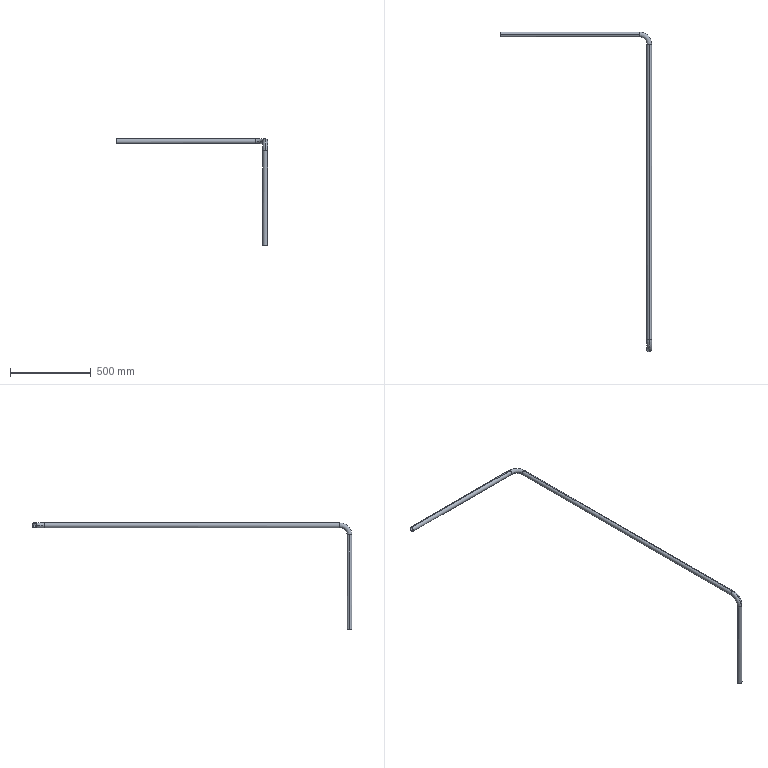Part | SolidWorks | features 3DProfileFeature 2, Sweep 1 | 1 solid | 22 faces | box 936.356 x 1980 x 658.195 mm | volume 609287 mm3 | cylinder 12 | torus 8 | plane 2 | commonest cylinder face diameters 26 x6 30 x6
STEP:
#1=CARTESIAN_POINT('',(750.,1143.697,-236.553));
#2=VERTEX_POINT('',#1);
#3=CARTESIAN_POINT('',(750.,1143.697,-210.553));
#4=VERTEX_POINT('',#3);
#5=CARTESIAN_POINT('',(750.,1143.697,-223.553));
#6=DIRECTION('',(0.,1.,0.));
#7=DIRECTION('',(0.,0.,-1.));
#8=AXIS2_PLACEMENT_3D('',#5,#6,#7);
#9=CIRCLE('',#8,13.);
#10=EDGE_CURVE('',#2,#4,#9,.T.);
#11=ORIENTED_EDGE('',*,*,#10,.T.);
#12=CARTESIAN_POINT('',(750.,1070.697,-283.553));
#13=VERTEX_POINT('',#12);
#14=CARTESIAN_POINT('',(750.,1143.697,-283.553));
#15=DIRECTION('',(1.,0.,0.));
#16=DIRECTION('',(0.,0.,-1.));
#17=AXIS2_PLACEMENT_3D('',#14,#15,#16);
#18=CIRCLE('',#17,73.);
#19=EDGE_CURVE('',#4,#13,#18,.T.);
#20=ORIENTED_EDGE('',*,*,#19,.T.);
#21=CARTESIAN_POINT('',(737.,1083.697,-283.553));
#22=VERTEX_POINT('',#21);
#23=CARTESIAN_POINT('',(750.,1083.697,-283.553));
#24=DIRECTION('',(0.,0.,1.));
#25=DIRECTION('',(0.,-1.,0.));
#26=AXIS2_PLACEMENT_3D('',#23,#24,#25);
#27=CIRCLE('',#26,13.);
#28=EDGE_CURVE('',#22,#13,#27,.T.);
#29=ORIENTED_EDGE('',*,*,#28,.F.);
#30=CARTESIAN_POINT('',(750.,1096.697,-283.553));
#31=VERTEX_POINT('',#30);
#32=CARTESIAN_POINT('',(750.,1083.697,-283.553));
#33=DIRECTION('',(0.,0.,1.));
#34=DIRECTION('',(0.,-1.,0.));
#35=AXIS2_PLACEMENT_3D('',#32,#33,#34);
#36=CIRCLE('',#35,13.);
#37=EDGE_CURVE('',#31,#22,#36,.T.);
#38=ORIENTED_EDGE('',*,*,#37,.F.);
#39=CARTESIAN_POINT('',(750.,1143.697,-283.553));
#40=DIRECTION('',(1.,0.,0.));
#41=DIRECTION('',(0.,0.,-1.));
#42=AXIS2_PLACEMENT_3D('',#39,#40,#41);
#43=CIRCLE('',#42,47.);
#44=EDGE_CURVE('',#2,#31,#43,.T.);
#45=ORIENTED_EDGE('',*,*,#44,.F.);
#46=EDGE_LOOP('',(#11,#20,#29,#38,#45));
#47=FACE_OUTER_BOUND('',#46,.T.);
#48=CARTESIAN_POINT('',(750.,1143.697,-283.553));
#49=DIRECTION('',(1.,0.,0.));
#50=DIRECTION('',(0.,0.,-1.));
#51=AXIS2_PLACEMENT_3D('',#48,#49,#50);
#52=TOROIDAL_SURFACE('',#51,60.,13.);
#53=ADVANCED_FACE('',(#47),#52,.F.);
#54=CARTESIAN_POINT('',(690.,3033.901,-210.553));
#55=VERTEX_POINT('',#54);
#56=CARTESIAN_POINT('',(690.,3046.901,-223.553));
#57=VERTEX_POINT('',#56);
#58=CARTESIAN_POINT('',(690.,3033.901,-223.553));
#59=DIRECTION('',(-1.,0.,0.));
#60=DIRECTION('',(0.,0.,-1.));
#61=AXIS2_PLACEMENT_3D('',#58,#59,#60);
#62=CIRCLE('',#61,13.);
#63=EDGE_CURVE('',#55,#57,#62,.T.);
#64=ORIENTED_EDGE('',*,*,#63,.T.);
#65=CARTESIAN_POINT('',(763.,2973.901,-223.553));
#66=VERTEX_POINT('',#65);
#67=CARTESIAN_POINT('',(690.,2973.901,-223.553));
#68=DIRECTION('',(0.,0.,-1.));
#69=DIRECTION('',(-1.,0.,0.));
#70=AXIS2_PLACEMENT_3D('',#67,#68,#69);
#71=CIRCLE('',#70,73.);
#72=EDGE_CURVE('',#57,#66,#71,.T.);
#73=ORIENTED_EDGE('',*,*,#72,.T.);
#74=CARTESIAN_POINT('',(750.,2973.901,-210.553));
#75=VERTEX_POINT('',#74);
#76=CARTESIAN_POINT('',(750.,2973.901,-223.553));
#77=DIRECTION('',(0.,1.,0.));
#78=DIRECTION('',(-1.,0.,0.));
#79=AXIS2_PLACEMENT_3D('',#76,#77,#78);
#80=CIRCLE('',#79,13.);
#81=EDGE_CURVE('',#75,#66,#80,.T.);
#82=ORIENTED_EDGE('',*,*,#81,.F.);
#83=CARTESIAN_POINT('',(737.,2973.901,-223.553));
#84=VERTEX_POINT('',#83);
#85=CARTESIAN_POINT('',(750.,2973.901,-223.553));
#86=DIRECTION('',(0.,1.,0.));
#87=DIRECTION('',(-1.,0.,0.));
#88=AXIS2_PLACEMENT_3D('',#85,#86,#87);
#89=CIRCLE('',#88,13.);
#90=EDGE_CURVE('',#84,#75,#89,.T.);
#91=ORIENTED_EDGE('',*,*,#90,.F.);
#92=CARTESIAN_POINT('',(690.,3020.901,-223.553));
#93=VERTEX_POINT('',#92);
#94=CARTESIAN_POINT('',(690.,2973.901,-223.553));
#95=DIRECTION('',(0.,0.,-1.));
#96=DIRECTION('',(-1.,0.,0.));
#97=AXIS2_PLACEMENT_3D('',#94,#95,#96);
#98=CIRCLE('',#97,47.);
#99=EDGE_CURVE('',#93,#84,#98,.T.);
#100=ORIENTED_EDGE('',*,*,#99,.F.);
#101=CARTESIAN_POINT('',(690.,3033.901,-223.553));
#102=DIRECTION('',(-1.,0.,0.));
#103=DIRECTION('',(0.,0.,-1.));
#104=AXIS2_PLACEMENT_3D('',#101,#102,#103);
#105=CIRCLE('',#104,13.);
#106=EDGE_CURVE('',#93,#55,#105,.T.);
#107=ORIENTED_EDGE('',*,*,#106,.T.);
#108=EDGE_LOOP('',(#64,#73,#82,#91,#100,#107));
#109=FACE_OUTER_BOUND('',#108,.T.);
#110=CARTESIAN_POINT('',(690.,2973.901,-223.553));
#111=DIRECTION('',(0.,0.,-1.));
#112=DIRECTION('',(-1.,0.,0.));
#113=AXIS2_PLACEMENT_3D('',#110,#111,#112);
#114=TOROIDAL_SURFACE('',#113,60.,13.);
#115=ADVANCED_FACE('',(#109),#114,.F.);
#116=CARTESIAN_POINT('',(750.,1143.697,-208.553));
#117=VERTEX_POINT('',#116);
#118=CARTESIAN_POINT('',(750.,1143.697,-238.553));
#119=VERTEX_POINT('',#118);
#120=CARTESIAN_POINT('',(750.,1143.697,-223.553));
#121=DIRECTION('',(0.,1.,0.));
#122=DIRECTION('',(1.,0.,0.));
#123=AXIS2_PLACEMENT_3D('',#120,#121,#122);
#124=CIRCLE('',#123,15.);
#125=EDGE_CURVE('',#117,#119,#124,.T.);
#126=ORIENTED_EDGE('',*,*,#125,.F.);
#127=CARTESIAN_POINT('',(750.,1068.697,-283.553));
#128=VERTEX_POINT('',#127);
#129=CARTESIAN_POINT('',(750.,1143.697,-283.553));
#130=DIRECTION('',(1.,0.,0.));
#131=DIRECTION('',(0.,0.,-1.));
#132=AXIS2_PLACEMENT_3D('',#129,#130,#131);
#133=CIRCLE('',#132,75.);
#134=EDGE_CURVE('',#117,#128,#133,.T.);
#135=ORIENTED_EDGE('',*,*,#134,.T.);
#136=CARTESIAN_POINT('',(765.,1083.697,-283.553));
#137=VERTEX_POINT('',#136);
#138=CARTESIAN_POINT('',(750.,1083.697,-283.553));
#139=DIRECTION('',(0.,0.,1.));
#140=DIRECTION('',(1.,0.,0.));
#141=AXIS2_PLACEMENT_3D('',#138,#139,#140);
#142=CIRCLE('',#141,15.);
#143=EDGE_CURVE('',#128,#137,#142,.T.);
#144=ORIENTED_EDGE('',*,*,#143,.T.);
#145=CARTESIAN_POINT('',(750.,1098.697,-283.553));
#146=VERTEX_POINT('',#145);
#147=CARTESIAN_POINT('',(750.,1083.697,-283.553));
#148=DIRECTION('',(0.,0.,1.));
#149=DIRECTION('',(1.,0.,0.));
#150=AXIS2_PLACEMENT_3D('',#147,#148,#149);
#151=CIRCLE('',#150,15.);
#152=EDGE_CURVE('',#137,#146,#151,.T.);
#153=ORIENTED_EDGE('',*,*,#152,.T.);
#154=CARTESIAN_POINT('',(750.,1143.697,-283.553));
#155=DIRECTION('',(1.,0.,0.));
#156=DIRECTION('',(0.,0.,-1.));
#157=AXIS2_PLACEMENT_3D('',#154,#155,#156);
#158=CIRCLE('',#157,45.);
#159=EDGE_CURVE('',#119,#146,#158,.T.);
#160=ORIENTED_EDGE('',*,*,#159,.F.);
#161=EDGE_LOOP('',(#126,#135,#144,#153,#160));
#162=FACE_OUTER_BOUND('',#161,.T.);
#163=CARTESIAN_POINT('',(750.,1143.697,-283.553));
#164=DIRECTION('',(1.,0.,0.));
#165=DIRECTION('',(0.,0.,-1.));
#166=AXIS2_PLACEMENT_3D('',#163,#164,#165);
#167=TOROIDAL_SURFACE('',#166,60.,15.);
#168=ADVANCED_FACE('',(#162),#167,.T.);
#169=CARTESIAN_POINT('',(690.,3048.901,-223.553));
#170=VERTEX_POINT('',#169);
#171=CARTESIAN_POINT('',(690.,3033.901,-238.553));
#172=VERTEX_POINT('',#171);
#173=CARTESIAN_POINT('',(690.,3033.901,-223.553));
#174=DIRECTION('',(-1.,0.,0.));
#175=DIRECTION('',(0.,1.,0.));
#176=AXIS2_PLACEMENT_3D('',#173,#174,#175);
#177=CIRCLE('',#176,15.);
#178=EDGE_CURVE('',#170,#172,#177,.T.);
#179=ORIENTED_EDGE('',*,*,#178,.F.);
#180=CARTESIAN_POINT('',(765.,2973.901,-223.553));
#181=VERTEX_POINT('',#180);
#182=CARTESIAN_POINT('',(690.,2973.901,-223.553));
#183=DIRECTION('',(0.,0.,-1.));
#184=DIRECTION('',(-1.,0.,0.));
#185=AXIS2_PLACEMENT_3D('',#182,#183,#184);
#186=CIRCLE('',#185,75.);
#187=EDGE_CURVE('',#170,#181,#186,.T.);
#188=ORIENTED_EDGE('',*,*,#187,.T.);
#189=CARTESIAN_POINT('',(750.,2973.901,-238.553));
#190=VERTEX_POINT('',#189);
#191=CARTESIAN_POINT('',(750.,2973.901,-223.553));
#192=DIRECTION('',(0.,1.,0.));
#193=DIRECTION('',(1.,0.,0.));
#194=AXIS2_PLACEMENT_3D('',#191,#192,#193);
#195=CIRCLE('',#194,15.);
#196=EDGE_CURVE('',#181,#190,#195,.T.);
#197=ORIENTED_EDGE('',*,*,#196,.T.);
#198=CARTESIAN_POINT('',(735.,2973.901,-223.553));
#199=VERTEX_POINT('',#198);
#200=CARTESIAN_POINT('',(750.,2973.901,-223.553));
#201=DIRECTION('',(0.,1.,0.));
#202=DIRECTION('',(1.,0.,0.));
#203=AXIS2_PLACEMENT_3D('',#200,#201,#202);
#204=CIRCLE('',#203,15.);
#205=EDGE_CURVE('',#190,#199,#204,.T.);
#206=ORIENTED_EDGE('',*,*,#205,.T.);
#207=CARTESIAN_POINT('',(690.,3018.901,-223.553));
#208=VERTEX_POINT('',#207);
#209=CARTESIAN_POINT('',(690.,2973.901,-223.553));
#210=DIRECTION('',(0.,0.,-1.));
#211=DIRECTION('',(-1.,0.,0.));
#212=AXIS2_PLACEMENT_3D('',#209,#210,#211);
#213=CIRCLE('',#212,45.);
#214=EDGE_CURVE('',#208,#199,#213,.T.);
#215=ORIENTED_EDGE('',*,*,#214,.F.);
#216=CARTESIAN_POINT('',(690.,3033.901,-223.553));
#217=DIRECTION('',(-1.,0.,0.));
#218=DIRECTION('',(0.,1.,0.));
#219=AXIS2_PLACEMENT_3D('',#216,#217,#218);
#220=CIRCLE('',#219,15.);
#221=EDGE_CURVE('',#172,#208,#220,.T.);
#222=ORIENTED_EDGE('',*,*,#221,.F.);
#223=EDGE_LOOP('',(#179,#188,#197,#206,#215,#222));
#224=FACE_OUTER_BOUND('',#223,.T.);
#225=CARTESIAN_POINT('',(690.,2973.901,-223.553));
#226=DIRECTION('',(0.,0.,-1.));
#227=DIRECTION('',(-1.,0.,0.));
#228=AXIS2_PLACEMENT_3D('',#225,#226,#227);
#229=TOROIDAL_SURFACE('',#228,60.,15.);
#230=ADVANCED_FACE('',(#224),#229,.T.);
#231=ORIENTED_EDGE('',*,*,#28,.T.);
#232=CARTESIAN_POINT('',(763.,1083.697,-283.553));
#233=VERTEX_POINT('',#232);
#234=CARTESIAN_POINT('',(750.,1083.697,-283.553));
#235=DIRECTION('',(0.,0.,1.));
#236=DIRECTION('',(0.,-1.,0.));
#237=AXIS2_PLACEMENT_3D('',#234,#235,#236);
#238=CIRCLE('',#237,13.);
#239=EDGE_CURVE('',#13,#233,#238,.T.);
#240=ORIENTED_EDGE('',*,*,#239,.T.);
#241=CARTESIAN_POINT('',(763.,1083.697,-866.748));
#242=VERTEX_POINT('',#241);
#243=CARTESIAN_POINT('',(763.,1083.697,-283.553));
#244=DIRECTION('',(0.,0.,-1.));
#245=VECTOR('',#244,1000.);
#246=LINE('',#243,#245);
#247=EDGE_CURVE('',#233,#242,#246,.T.);
#248=ORIENTED_EDGE('',*,*,#247,.T.);
#249=CARTESIAN_POINT('',(737.,1083.697,-866.748));
#250=VERTEX_POINT('',#249);
#251=CARTESIAN_POINT('',(750.,1083.697,-866.748));
#252=DIRECTION('',(0.,0.,1.));
#253=DIRECTION('',(1.,0.,0.));
#254=AXIS2_PLACEMENT_3D('',#251,#252,#253);
#255=CIRCLE('',#254,13.);
#256=EDGE_CURVE('',#250,#242,#255,.T.);
#257=ORIENTED_EDGE('',*,*,#256,.F.);
#258=CARTESIAN_POINT('',(737.,1083.697,-283.553));
#259=DIRECTION('',(0.,0.,-1.));
#260=VECTOR('',#259,1000.);
#261=LINE('',#258,#260);
#262=EDGE_CURVE('',#22,#250,#261,.T.);
#263=ORIENTED_EDGE('',*,*,#262,.F.);
#264=EDGE_LOOP('',(#231,#240,#248,#257,#263));
#265=FACE_OUTER_BOUND('',#264,.T.);
#266=CARTESIAN_POINT('',(750.,1083.697,-283.553));
#267=DIRECTION('',(0.,0.,-1.));
#268=DIRECTION('',(-1.,0.,0.));
#269=AXIS2_PLACEMENT_3D('',#266,#267,#268);
#270=CYLINDRICAL_SURFACE('',#269,13.);
#271=ADVANCED_FACE('',(#265),#270,.F.);
#272=CARTESIAN_POINT('',(750.,2973.901,-236.553));
#273=VERTEX_POINT('',#272);
#274=CARTESIAN_POINT('',(750.,2973.901,-223.553));
#275=DIRECTION('',(0.,1.,0.));
#276=DIRECTION('',(-1.,0.,0.));
#277=AXIS2_PLACEMENT_3D('',#274,#275,#276);
#278=CIRCLE('',#277,13.);
#279=EDGE_CURVE('',#273,#84,#278,.T.);
#280=ORIENTED_EDGE('',*,*,#279,.T.);
#281=ORIENTED_EDGE('',*,*,#90,.T.);
#282=CARTESIAN_POINT('',(750.,2973.901,-210.553));
#283=DIRECTION('',(0.,-1.,0.));
#284=VECTOR('',#283,1000.);
#285=LINE('',#282,#284);
#286=EDGE_CURVE('',#75,#4,#285,.T.);
#287=ORIENTED_EDGE('',*,*,#286,.T.);
#288=ORIENTED_EDGE('',*,*,#10,.F.);
#289=CARTESIAN_POINT('',(750.,2973.901,-236.553));
#290=DIRECTION('',(0.,-1.,0.));
#291=VECTOR('',#290,1000.);
#292=LINE('',#289,#291);
#293=EDGE_CURVE('',#273,#2,#292,.T.);
#294=ORIENTED_EDGE('',*,*,#293,.F.);
#295=EDGE_LOOP('',(#280,#281,#287,#288,#294));
#296=FACE_OUTER_BOUND('',#295,.T.);
#297=CARTESIAN_POINT('',(750.,2973.901,-223.553));
#298=DIRECTION('',(0.,-1.,0.));
#299=DIRECTION('',(0.,0.,-1.));
#300=AXIS2_PLACEMENT_3D('',#297,#298,#299);
#301=CYLINDRICAL_SURFACE('',#300,13.);
#302=ADVANCED_FACE('',(#296),#301,.F.);
#303=CARTESIAN_POINT('',(-171.356,3033.901,-236.553));
#304=VERTEX_POINT('',#303);
#305=CARTESIAN_POINT('',(-171.356,3033.901,-210.553));
#306=VERTEX_POINT('',#305);
#307=CARTESIAN_POINT('',(-171.356,3033.901,-223.553));
#308=DIRECTION('',(-1.,0.,0.));
#309=DIRECTION('',(0.,0.,1.));
#310=AXIS2_PLACEMENT_3D('',#307,#308,#309);
#311=CIRCLE('',#310,13.);
#312=EDGE_CURVE('',#304,#306,#311,.T.);
#313=ORIENTED_EDGE('',*,*,#312,.T.);
#314=CARTESIAN_POINT('',(-171.356,3033.901,-210.553));
#315=DIRECTION('',(1.,0.,0.));
#316=VECTOR('',#315,1000.);
#317=LINE('',#314,#316);
#318=EDGE_CURVE('',#306,#55,#317,.T.);
#319=ORIENTED_EDGE('',*,*,#318,.T.);
#320=ORIENTED_EDGE('',*,*,#106,.F.);
#321=CARTESIAN_POINT('',(690.,3033.901,-236.553));
#322=VERTEX_POINT('',#321);
#323=CARTESIAN_POINT('',(690.,3033.901,-223.553));
#324=DIRECTION('',(-1.,0.,0.));
#325=DIRECTION('',(0.,0.,-1.));
#326=AXIS2_PLACEMENT_3D('',#323,#324,#325);
#327=CIRCLE('',#326,13.);
#328=EDGE_CURVE('',#322,#93,#327,.T.);
#329=ORIENTED_EDGE('',*,*,#328,.F.);
#330=CARTESIAN_POINT('',(-171.356,3033.901,-236.553));
#331=DIRECTION('',(1.,0.,0.));
#332=VECTOR('',#331,1000.);
#333=LINE('',#330,#332);
#334=EDGE_CURVE('',#304,#322,#333,.T.);
#335=ORIENTED_EDGE('',*,*,#334,.F.);
#336=EDGE_LOOP('',(#313,#319,#320,#329,#335));
#337=FACE_OUTER_BOUND('',#336,.T.);
#338=CARTESIAN_POINT('',(-171.356,3033.901,-223.553));
#339=DIRECTION('',(1.,0.,0.));
#340=DIRECTION('',(0.,0.,-1.));
#341=AXIS2_PLACEMENT_3D('',#338,#339,#340);
#342=CYLINDRICAL_SURFACE('',#341,13.);
#343=ADVANCED_FACE('',(#337),#342,.F.);
#344=ORIENTED_EDGE('',*,*,#152,.F.);
#345=CARTESIAN_POINT('',(765.,1083.697,-866.748));
#346=VERTEX_POINT('',#345);
#347=CARTESIAN_POINT('',(765.,1083.697,-283.553));
#348=DIRECTION('',(0.,0.,-1.));
#349=VECTOR('',#348,1000.);
#350=LINE('',#347,#349);
#351=EDGE_CURVE('',#137,#346,#350,.T.);
#352=ORIENTED_EDGE('',*,*,#351,.T.);
#353=CARTESIAN_POINT('',(735.,1083.697,-866.748));
#354=VERTEX_POINT('',#353);
#355=CARTESIAN_POINT('',(750.,1083.697,-866.748));
#356=DIRECTION('',(0.,0.,1.));
#357=DIRECTION('',(1.,0.,0.));
#358=AXIS2_PLACEMENT_3D('',#355,#356,#357);
#359=CIRCLE('',#358,15.);
#360=EDGE_CURVE('',#346,#354,#359,.T.);
#361=ORIENTED_EDGE('',*,*,#360,.T.);
#362=CARTESIAN_POINT('',(735.,1083.697,-283.553));
#363=VERTEX_POINT('',#362);
#364=CARTESIAN_POINT('',(735.,1083.697,-283.553));
#365=DIRECTION('',(0.,0.,-1.));
#366=VECTOR('',#365,1000.);
#367=LINE('',#364,#366);
#368=EDGE_CURVE('',#363,#354,#367,.T.);
#369=ORIENTED_EDGE('',*,*,#368,.F.);
#370=CARTESIAN_POINT('',(750.,1083.697,-283.553));
#371=DIRECTION('',(0.,0.,1.));
#372=DIRECTION('',(1.,0.,0.));
#373=AXIS2_PLACEMENT_3D('',#370,#371,#372);
#374=CIRCLE('',#373,15.);
#375=EDGE_CURVE('',#146,#363,#374,.T.);
#376=ORIENTED_EDGE('',*,*,#375,.F.);
#377=EDGE_LOOP('',(#344,#352,#361,#369,#376));
#378=FACE_OUTER_BOUND('',#377,.T.);
#379=CARTESIAN_POINT('',(750.,1083.697,-283.553));
#380=DIRECTION('',(0.,0.,-1.));
#381=DIRECTION('',(-1.,0.,0.));
#382=AXIS2_PLACEMENT_3D('',#379,#380,#381);
#383=CYLINDRICAL_SURFACE('',#382,15.);
#384=ADVANCED_FACE('',(#378),#383,.T.);
#385=CARTESIAN_POINT('',(750.,2973.901,-208.553));
#386=VERTEX_POINT('',#385);
#387=CARTESIAN_POINT('',(750.,2973.901,-223.553));
#388=DIRECTION('',(0.,1.,0.));
#389=DIRECTION('',(1.,0.,0.));
#390=AXIS2_PLACEMENT_3D('',#387,#388,#389);
#391=CIRCLE('',#390,15.);
#392=EDGE_CURVE('',#386,#181,#391,.T.);
#393=ORIENTED_EDGE('',*,*,#392,.F.);
#394=CARTESIAN_POINT('',(750.,2973.901,-208.553));
#395=DIRECTION('',(0.,-1.,0.));
#396=VECTOR('',#395,1000.);
#397=LINE('',#394,#396);
#398=EDGE_CURVE('',#386,#117,#397,.T.);
#399=ORIENTED_EDGE('',*,*,#398,.T.);
#400=ORIENTED_EDGE('',*,*,#125,.T.);
#401=CARTESIAN_POINT('',(750.,2973.901,-238.553));
#402=DIRECTION('',(0.,-1.,0.));
#403=VECTOR('',#402,1000.);
#404=LINE('',#401,#403);
#405=EDGE_CURVE('',#190,#119,#404,.T.);
#406=ORIENTED_EDGE('',*,*,#405,.F.);
#407=ORIENTED_EDGE('',*,*,#196,.F.);
#408=EDGE_LOOP('',(#393,#399,#400,#406,#407));
#409=FACE_OUTER_BOUND('',#408,.T.);
#410=CARTESIAN_POINT('',(750.,2973.901,-223.553));
#411=DIRECTION('',(0.,-1.,0.));
#412=DIRECTION('',(0.,0.,-1.));
#413=AXIS2_PLACEMENT_3D('',#410,#411,#412);
#414=CYLINDRICAL_SURFACE('',#413,15.);
#415=ADVANCED_FACE('',(#409),#414,.T.);
#416=CARTESIAN_POINT('',(-171.356,3033.901,-208.553));
#417=VERTEX_POINT('',#416);
#418=CARTESIAN_POINT('',(-171.356,3033.901,-238.553));
#419=VERTEX_POINT('',#418);
#420=CARTESIAN_POINT('',(-171.356,3033.901,-223.553));
#421=DIRECTION('',(-1.,0.,0.));
#422=DIRECTION('',(0.,1.,0.));
#423=AXIS2_PLACEMENT_3D('',#420,#421,#422);
#424=CIRCLE('',#423,15.);
#425=EDGE_CURVE('',#417,#419,#424,.T.);
#426=ORIENTED_EDGE('',*,*,#425,.F.);
#427=CARTESIAN_POINT('',(690.,3033.901,-208.553));
#428=VERTEX_POINT('',#427);
#429=CARTESIAN_POINT('',(-171.356,3033.901,-208.553));
#430=DIRECTION('',(1.,0.,0.));
#431=VECTOR('',#430,1000.);
#432=LINE('',#429,#431);
#433=EDGE_CURVE('',#417,#428,#432,.T.);
#434=ORIENTED_EDGE('',*,*,#433,.T.);
#435=CARTESIAN_POINT('',(690.,3033.901,-223.553));
#436=DIRECTION('',(-1.,0.,0.));
#437=DIRECTION('',(0.,1.,0.));
#438=AXIS2_PLACEMENT_3D('',#435,#436,#437);
#439=CIRCLE('',#438,15.);
#440=EDGE_CURVE('',#428,#170,#439,.T.);
#441=ORIENTED_EDGE('',*,*,#440,.T.);
#442=ORIENTED_EDGE('',*,*,#178,.T.);
#443=CARTESIAN_POINT('',(-171.356,3033.901,-238.553));
#444=DIRECTION('',(1.,0.,0.));
#445=VECTOR('',#444,1000.);
#446=LINE('',#443,#445);
#447=EDGE_CURVE('',#419,#172,#446,.T.);
#448=ORIENTED_EDGE('',*,*,#447,.F.);
#449=EDGE_LOOP('',(#426,#434,#441,#442,#448));
#450=FACE_OUTER_BOUND('',#449,.T.);
#451=CARTESIAN_POINT('',(-171.356,3033.901,-223.553));
#452=DIRECTION('',(1.,0.,0.));
#453=DIRECTION('',(0.,0.,-1.));
#454=AXIS2_PLACEMENT_3D('',#451,#452,#453);
#455=CYLINDRICAL_SURFACE('',#454,15.);
#456=ADVANCED_FACE('',(#450),#455,.T.);
#457=ORIENTED_EDGE('',*,*,#351,.F.);
#458=ORIENTED_EDGE('',*,*,#143,.F.);
#459=CARTESIAN_POINT('',(750.,1083.697,-283.553));
#460=DIRECTION('',(0.,0.,1.));
#461=DIRECTION('',(1.,0.,0.));
#462=AXIS2_PLACEMENT_3D('',#459,#460,#461);
#463=CIRCLE('',#462,15.);
#464=EDGE_CURVE('',#363,#128,#463,.T.);
#465=ORIENTED_EDGE('',*,*,#464,.F.);
#466=ORIENTED_EDGE('',*,*,#368,.T.);
#467=CARTESIAN_POINT('',(750.,1083.697,-866.748));
#468=DIRECTION('',(0.,0.,1.));
#469=DIRECTION('',(1.,0.,0.));
#470=AXIS2_PLACEMENT_3D('',#467,#468,#469);
#471=CIRCLE('',#470,15.);
#472=EDGE_CURVE('',#354,#346,#471,.T.);
#473=ORIENTED_EDGE('',*,*,#472,.T.);
#474=EDGE_LOOP('',(#457,#458,#465,#466,#473));
#475=FACE_OUTER_BOUND('',#474,.T.);
#476=CARTESIAN_POINT('',(750.,1083.697,-283.553));
#477=DIRECTION('',(0.,0.,-1.));
#478=DIRECTION('',(-1.,0.,0.));
#479=AXIS2_PLACEMENT_3D('',#476,#477,#478);
#480=CYLINDRICAL_SURFACE('',#479,15.);
#481=ADVANCED_FACE('',(#475),#480,.T.);
#482=ORIENTED_EDGE('',*,*,#134,.F.);
#483=CARTESIAN_POINT('',(750.,1143.697,-223.553));
#484=DIRECTION('',(0.,1.,0.));
#485=DIRECTION('',(1.,0.,0.));
#486=AXIS2_PLACEMENT_3D('',#483,#484,#485);
#487=CIRCLE('',#486,15.);
#488=EDGE_CURVE('',#119,#117,#487,.T.);
#489=ORIENTED_EDGE('',*,*,#488,.F.);
#490=ORIENTED_EDGE('',*,*,#159,.T.);
#491=ORIENTED_EDGE('',*,*,#375,.T.);
#492=ORIENTED_EDGE('',*,*,#464,.T.);
#493=EDGE_LOOP('',(#482,#489,#490,#491,#492));
#494=FACE_OUTER_BOUND('',#493,.T.);
#495=CARTESIAN_POINT('',(750.,1143.697,-283.553));
#496=DIRECTION('',(1.,0.,0.));
#497=DIRECTION('',(0.,0.,-1.));
#498=AXIS2_PLACEMENT_3D('',#495,#496,#497);
#499=TOROIDAL_SURFACE('',#498,60.,15.);
#500=ADVANCED_FACE('',(#494),#499,.T.);
#501=ORIENTED_EDGE('',*,*,#398,.F.);
#502=CARTESIAN_POINT('',(750.,2973.901,-223.553));
#503=DIRECTION('',(0.,1.,0.));
#504=DIRECTION('',(1.,0.,0.));
#505=AXIS2_PLACEMENT_3D('',#502,#503,#504);
#506=CIRCLE('',#505,15.);
#507=EDGE_CURVE('',#199,#386,#506,.T.);
#508=ORIENTED_EDGE('',*,*,#507,.F.);
#509=ORIENTED_EDGE('',*,*,#205,.F.);
#510=ORIENTED_EDGE('',*,*,#405,.T.);
#511=ORIENTED_EDGE('',*,*,#488,.T.);
#512=EDGE_LOOP('',(#501,#508,#509,#510,#511));
#513=FACE_OUTER_BOUND('',#512,.T.);
#514=CARTESIAN_POINT('',(750.,2973.901,-223.553));
#515=DIRECTION('',(0.,-1.,0.));
#516=DIRECTION('',(0.,0.,-1.));
#517=AXIS2_PLACEMENT_3D('',#514,#515,#516);
#518=CYLINDRICAL_SURFACE('',#517,15.);
#519=ADVANCED_FACE('',(#513),#518,.T.);
#520=ORIENTED_EDGE('',*,*,#187,.F.);
#521=ORIENTED_EDGE('',*,*,#440,.F.);
#522=CARTESIAN_POINT('',(690.,3033.901,-223.553));
#523=DIRECTION('',(-1.,0.,0.));
#524=DIRECTION('',(0.,1.,0.));
#525=AXIS2_PLACEMENT_3D('',#522,#523,#524);
#526=CIRCLE('',#525,15.);
#527=EDGE_CURVE('',#208,#428,#526,.T.);
#528=ORIENTED_EDGE('',*,*,#527,.F.);
#529=ORIENTED_EDGE('',*,*,#214,.T.);
#530=ORIENTED_EDGE('',*,*,#507,.T.);
#531=ORIENTED_EDGE('',*,*,#392,.T.);
#532=EDGE_LOOP('',(#520,#521,#528,#529,#530,#531));
#533=FACE_OUTER_BOUND('',#532,.T.);
#534=CARTESIAN_POINT('',(690.,2973.901,-223.553));
#535=DIRECTION('',(0.,0.,-1.));
#536=DIRECTION('',(-1.,0.,0.));
#537=AXIS2_PLACEMENT_3D('',#534,#535,#536);
#538=TOROIDAL_SURFACE('',#537,60.,15.);
#539=ADVANCED_FACE('',(#533),#538,.T.);
#540=ORIENTED_EDGE('',*,*,#433,.F.);
#541=CARTESIAN_POINT('',(-171.356,3033.901,-223.553));
#542=DIRECTION('',(-1.,0.,0.));
#543=DIRECTION('',(0.,1.,0.));
#544=AXIS2_PLACEMENT_3D('',#541,#542,#543);
#545=CIRCLE('',#544,15.);
#546=EDGE_CURVE('',#419,#417,#545,.T.);
#547=ORIENTED_EDGE('',*,*,#546,.F.);
#548=ORIENTED_EDGE('',*,*,#447,.T.);
#549=ORIENTED_EDGE('',*,*,#221,.T.);
#550=ORIENTED_EDGE('',*,*,#527,.T.);
#551=EDGE_LOOP('',(#540,#547,#548,#549,#550));
#552=FACE_OUTER_BOUND('',#551,.T.);
#553=CARTESIAN_POINT('',(-171.356,3033.901,-223.553));
#554=DIRECTION('',(1.,0.,0.));
#555=DIRECTION('',(0.,0.,-1.));
#556=AXIS2_PLACEMENT_3D('',#553,#554,#555);
#557=CYLINDRICAL_SURFACE('',#556,15.);
#558=ADVANCED_FACE('',(#552),#557,.T.);
#559=ORIENTED_EDGE('',*,*,#256,.T.);
#560=CARTESIAN_POINT('',(750.,1083.697,-866.748));
#561=DIRECTION('',(0.,0.,1.));
#562=DIRECTION('',(1.,0.,0.));
#563=AXIS2_PLACEMENT_3D('',#560,#561,#562);
#564=CIRCLE('',#563,13.);
#565=EDGE_CURVE('',#242,#250,#564,.T.);
#566=ORIENTED_EDGE('',*,*,#565,.T.);
#567=EDGE_LOOP('',(#559,#566));
#568=FACE_BOUND('',#567,.T.);
#569=ORIENTED_EDGE('',*,*,#472,.F.);
#570=ORIENTED_EDGE('',*,*,#360,.F.);
#571=EDGE_LOOP('',(#569,#570));
#572=FACE_OUTER_BOUND('',#571,.T.);
#573=CARTESIAN_POINT('',(750.,1083.697,-866.748));
#574=DIRECTION('',(0.,0.,1.));
#575=DIRECTION('',(1.,0.,0.));
#576=AXIS2_PLACEMENT_3D('',#573,#574,#575);
#577=PLANE('',#576);
#578=ADVANCED_FACE('',(#568,#572),#577,.F.);
#579=ORIENTED_EDGE('',*,*,#312,.F.);
#580=CARTESIAN_POINT('',(-171.356,3033.901,-223.553));
#581=DIRECTION('',(-1.,0.,0.));
#582=DIRECTION('',(0.,0.,1.));
#583=AXIS2_PLACEMENT_3D('',#580,#581,#582);
#584=CIRCLE('',#583,13.);
#585=EDGE_CURVE('',#306,#304,#584,.T.);
#586=ORIENTED_EDGE('',*,*,#585,.F.);
#587=EDGE_LOOP('',(#579,#586));
#588=FACE_BOUND('',#587,.T.);
#589=ORIENTED_EDGE('',*,*,#546,.T.);
#590=ORIENTED_EDGE('',*,*,#425,.T.);
#591=EDGE_LOOP('',(#589,#590));
#592=FACE_OUTER_BOUND('',#591,.T.);
#593=CARTESIAN_POINT('',(-171.356,3033.901,-223.553));
#594=DIRECTION('',(-1.,0.,0.));
#595=DIRECTION('',(0.,1.,0.));
#596=AXIS2_PLACEMENT_3D('',#593,#594,#595);
#597=PLANE('',#596);
#598=ADVANCED_FACE('',(#588,#592),#597,.T.);
#599=ORIENTED_EDGE('',*,*,#247,.F.);
#600=CARTESIAN_POINT('',(750.,1083.697,-283.553));
#601=DIRECTION('',(0.,0.,1.));
#602=DIRECTION('',(0.,-1.,0.));
#603=AXIS2_PLACEMENT_3D('',#600,#601,#602);
#604=CIRCLE('',#603,13.);
#605=EDGE_CURVE('',#233,#31,#604,.T.);
#606=ORIENTED_EDGE('',*,*,#605,.T.);
#607=ORIENTED_EDGE('',*,*,#37,.T.);
#608=ORIENTED_EDGE('',*,*,#262,.T.);
#609=ORIENTED_EDGE('',*,*,#565,.F.);
#610=EDGE_LOOP('',(#599,#606,#607,#608,#609));
#611=FACE_OUTER_BOUND('',#610,.T.);
#612=CARTESIAN_POINT('',(750.,1083.697,-283.553));
#613=DIRECTION('',(0.,0.,-1.));
#614=DIRECTION('',(-1.,0.,0.));
#615=AXIS2_PLACEMENT_3D('',#612,#613,#614);
#616=CYLINDRICAL_SURFACE('',#615,13.);
#617=ADVANCED_FACE('',(#611),#616,.F.);
#618=ORIENTED_EDGE('',*,*,#19,.F.);
#619=CARTESIAN_POINT('',(750.,1143.697,-223.553));
#620=DIRECTION('',(0.,1.,0.));
#621=DIRECTION('',(0.,0.,-1.));
#622=AXIS2_PLACEMENT_3D('',#619,#620,#621);
#623=CIRCLE('',#622,13.);
#624=EDGE_CURVE('',#4,#2,#623,.T.);
#625=ORIENTED_EDGE('',*,*,#624,.T.);
#626=ORIENTED_EDGE('',*,*,#44,.T.);
#627=ORIENTED_EDGE('',*,*,#605,.F.);
#628=ORIENTED_EDGE('',*,*,#239,.F.);
#629=EDGE_LOOP('',(#618,#625,#626,#627,#628));
#630=FACE_OUTER_BOUND('',#629,.T.);
#631=CARTESIAN_POINT('',(750.,1143.697,-283.553));
#632=DIRECTION('',(1.,0.,0.));
#633=DIRECTION('',(0.,0.,-1.));
#634=AXIS2_PLACEMENT_3D('',#631,#632,#633);
#635=TOROIDAL_SURFACE('',#634,60.,13.);
#636=ADVANCED_FACE('',(#630),#635,.F.);
#637=ORIENTED_EDGE('',*,*,#286,.F.);
#638=ORIENTED_EDGE('',*,*,#81,.T.);
#639=CARTESIAN_POINT('',(750.,2973.901,-223.553));
#640=DIRECTION('',(0.,1.,0.));
#641=DIRECTION('',(-1.,0.,0.));
#642=AXIS2_PLACEMENT_3D('',#639,#640,#641);
#643=CIRCLE('',#642,13.);
#644=EDGE_CURVE('',#66,#273,#643,.T.);
#645=ORIENTED_EDGE('',*,*,#644,.T.);
#646=ORIENTED_EDGE('',*,*,#293,.T.);
#647=ORIENTED_EDGE('',*,*,#624,.F.);
#648=EDGE_LOOP('',(#637,#638,#645,#646,#647));
#649=FACE_OUTER_BOUND('',#648,.T.);
#650=CARTESIAN_POINT('',(750.,2973.901,-223.553));
#651=DIRECTION('',(0.,-1.,0.));
#652=DIRECTION('',(0.,0.,-1.));
#653=AXIS2_PLACEMENT_3D('',#650,#651,#652);
#654=CYLINDRICAL_SURFACE('',#653,13.);
#655=ADVANCED_FACE('',(#649),#654,.F.);
#656=ORIENTED_EDGE('',*,*,#72,.F.);
#657=CARTESIAN_POINT('',(690.,3033.901,-223.553));
#658=DIRECTION('',(-1.,0.,0.));
#659=DIRECTION('',(0.,0.,-1.));
#660=AXIS2_PLACEMENT_3D('',#657,#658,#659);
#661=CIRCLE('',#660,13.);
#662=EDGE_CURVE('',#57,#322,#661,.T.);
#663=ORIENTED_EDGE('',*,*,#662,.T.);
#664=ORIENTED_EDGE('',*,*,#328,.T.);
#665=ORIENTED_EDGE('',*,*,#99,.T.);
#666=ORIENTED_EDGE('',*,*,#279,.F.);
#667=ORIENTED_EDGE('',*,*,#644,.F.);
#668=EDGE_LOOP('',(#656,#663,#664,#665,#666,#667));
#669=FACE_OUTER_BOUND('',#668,.T.);
#670=CARTESIAN_POINT('',(690.,2973.901,-223.553));
#671=DIRECTION('',(0.,0.,-1.));
#672=DIRECTION('',(-1.,0.,0.));
#673=AXIS2_PLACEMENT_3D('',#670,#671,#672);
#674=TOROIDAL_SURFACE('',#673,60.,13.);
#675=ADVANCED_FACE('',(#669),#674,.F.);
#676=ORIENTED_EDGE('',*,*,#318,.F.);
#677=ORIENTED_EDGE('',*,*,#585,.T.);
#678=ORIENTED_EDGE('',*,*,#334,.T.);
#679=ORIENTED_EDGE('',*,*,#662,.F.);
#680=ORIENTED_EDGE('',*,*,#63,.F.);
#681=EDGE_LOOP('',(#676,#677,#678,#679,#680));
#682=FACE_OUTER_BOUND('',#681,.T.);
#683=CARTESIAN_POINT('',(-171.356,3033.901,-223.553));
#684=DIRECTION('',(1.,0.,0.));
#685=DIRECTION('',(0.,0.,-1.));
#686=AXIS2_PLACEMENT_3D('',#683,#684,#685);
#687=CYLINDRICAL_SURFACE('',#686,13.);
#688=ADVANCED_FACE('',(#682),#687,.F.);
#689=CLOSED_SHELL('',(#53,#115,#168,#230,#271,#302,#343,#384,#415,#456,#481,#500,#519,#539,#558,#578,#598,#617,#636,#655,#675,#688));
#690=MANIFOLD_SOLID_BREP('',#689);
#691=CARTESIAN_POINT('',(0.,0.,0.));
#692=DIRECTION('',(0.,0.,1.));
#693=DIRECTION('',(1.,0.,0.));
#694=AXIS2_PLACEMENT_3D('',#691,#692,#693);
#695=(LENGTH_UNIT()NAMED_UNIT(*)SI_UNIT(.MILLI.,.METRE.));
#696=UNCERTAINTY_MEASURE_WITH_UNIT(LENGTH_MEASURE(0.00001),#695,'','');
#697=(NAMED_UNIT(*)PLANE_ANGLE_UNIT()SI_UNIT($,.RADIAN.));
#698=(NAMED_UNIT(*)SI_UNIT($,.STERADIAN.)SOLID_ANGLE_UNIT());
#699=(GEOMETRIC_REPRESENTATION_CONTEXT(3)GLOBAL_UNCERTAINTY_ASSIGNED_CONTEXT((#696))GLOBAL_UNIT_ASSIGNED_CONTEXT((#695,#697,#698))REPRESENTATION_CONTEXT('',''));
#700=ADVANCED_BREP_SHAPE_REPRESENTATION('',(#690,#694),#699);